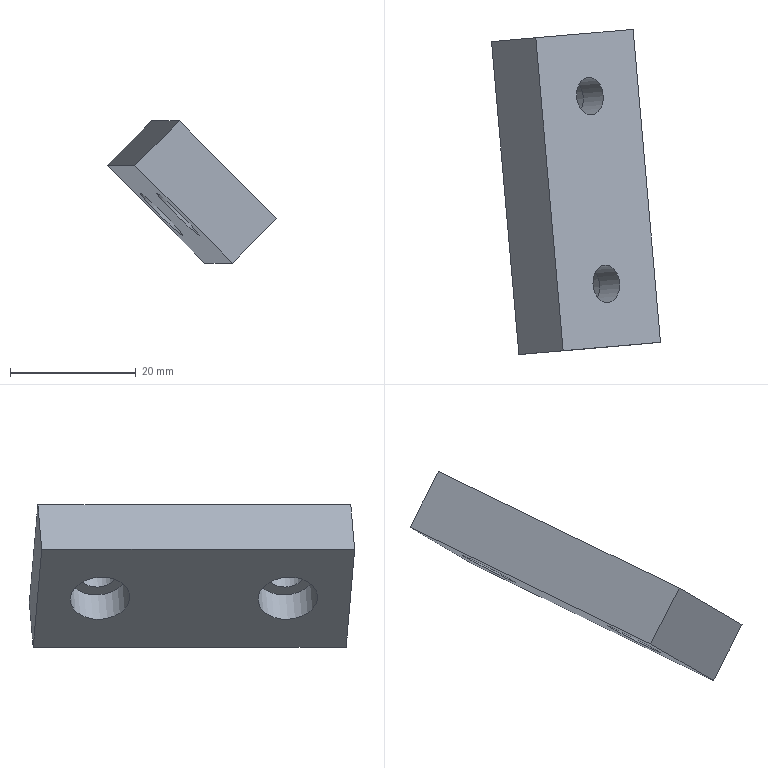Part | NX | features solid 2 | 1 solid | 12 faces | box 26.899 x 51.782 x 22.627 mm | volume 9966 mm3 | plane 8 | cylinder 4 | commonest cylinder face diameters 6 x2 9.5 x2
STEP:
#1=CARTESIAN_POINT('',(-359.245,41.849,8.934));
#2=VERTEX_POINT('',#1);
#3=CARTESIAN_POINT('',(-366.289,41.233,1.863));
#4=VERTEX_POINT('',#3);
#5=CARTESIAN_POINT('',(-359.245,41.849,8.934));
#6=DIRECTION('',(0.7044,0.06163,0.7071));
#7=VECTOR('',#6,1000.);
#8=LINE('',#5,#7);
#9=EDGE_CURVE('',#2,#4,#8,.F.);
#10=ORIENTED_EDGE('',*,*,#9,.F.);
#11=CARTESIAN_POINT('',(-354.887,-7.961,8.934));
#12=VERTEX_POINT('',#11);
#13=CARTESIAN_POINT('',(-359.463,44.34,8.934));
#14=DIRECTION('',(0.08716,-0.9962,0.));
#15=VECTOR('',#14,1000.);
#16=LINE('',#13,#15);
#17=EDGE_CURVE('',#2,#12,#16,.T.);
#18=ORIENTED_EDGE('',*,*,#17,.T.);
#19=CARTESIAN_POINT('',(-361.931,-8.577,1.863));
#20=VERTEX_POINT('',#19);
#21=CARTESIAN_POINT('',(-354.887,-7.961,8.934));
#22=DIRECTION('',(-0.7044,-0.06163,-0.7071));
#23=VECTOR('',#22,1000.);
#24=LINE('',#21,#23);
#25=EDGE_CURVE('',#12,#20,#24,.T.);
#26=ORIENTED_EDGE('',*,*,#25,.T.);
#27=CARTESIAN_POINT('',(-366.507,43.723,1.863));
#28=DIRECTION('',(0.08716,-0.9962,0.));
#29=VECTOR('',#28,1000.);
#30=LINE('',#27,#29);
#31=EDGE_CURVE('',#4,#20,#30,.T.);
#32=ORIENTED_EDGE('',*,*,#31,.F.);
#33=EDGE_LOOP('',(#10,#18,#26,#32));
#34=FACE_BOUND('',#33,.T.);
#35=CARTESIAN_POINT('',(-359.463,44.34,8.934));
#36=DIRECTION('',(0.7044,0.06163,-0.7071));
#37=DIRECTION('',(0.08716,-0.9962,0.));
#38=AXIS2_PLACEMENT_3D('',#35,#36,#37);
#39=PLANE('',#38);
#40=ADVANCED_FACE('',(#34),#39,.T.);
#41=ORIENTED_EDGE('',*,*,#25,.F.);
#42=CARTESIAN_POINT('',(-370.384,-9.317,24.49));
#43=VERTEX_POINT('',#42);
#44=CARTESIAN_POINT('',(-354.887,-7.961,8.934));
#45=DIRECTION('',(-0.7044,-0.06163,0.7071));
#46=VECTOR('',#45,1000.);
#47=LINE('',#44,#46);
#48=EDGE_CURVE('',#12,#43,#47,.T.);
#49=ORIENTED_EDGE('',*,*,#48,.T.);
#50=CARTESIAN_POINT('',(-377.428,-9.933,17.419));
#51=VERTEX_POINT('',#50);
#52=CARTESIAN_POINT('',(-370.384,-9.317,24.49));
#53=DIRECTION('',(0.7044,0.06163,0.7071));
#54=VECTOR('',#53,1000.);
#55=LINE('',#52,#54);
#56=EDGE_CURVE('',#43,#51,#55,.F.);
#57=ORIENTED_EDGE('',*,*,#56,.T.);
#58=CARTESIAN_POINT('',(-361.931,-8.577,1.863));
#59=DIRECTION('',(-0.7044,-0.06163,0.7071));
#60=VECTOR('',#59,1000.);
#61=LINE('',#58,#60);
#62=EDGE_CURVE('',#20,#51,#61,.T.);
#63=ORIENTED_EDGE('',*,*,#62,.F.);
#64=EDGE_LOOP('',(#41,#49,#57,#63));
#65=FACE_BOUND('',#64,.T.);
#66=CARTESIAN_POINT('',(-354.887,-7.961,8.934));
#67=DIRECTION('',(0.08716,-0.9962,0.));
#68=DIRECTION('',(-0.7044,-0.06163,0.7071));
#69=AXIS2_PLACEMENT_3D('',#66,#67,#68);
#70=PLANE('',#69);
#71=ADVANCED_FACE('',(#65),#70,.T.);
#72=ORIENTED_EDGE('',*,*,#56,.F.);
#73=CARTESIAN_POINT('',(-374.742,40.493,24.49));
#74=VERTEX_POINT('',#73);
#75=CARTESIAN_POINT('',(-374.96,42.984,24.49));
#76=DIRECTION('',(0.08716,-0.9962,0.));
#77=VECTOR('',#76,1000.);
#78=LINE('',#75,#77);
#79=EDGE_CURVE('',#74,#43,#78,.T.);
#80=ORIENTED_EDGE('',*,*,#79,.F.);
#81=CARTESIAN_POINT('',(-381.786,39.877,17.419));
#82=VERTEX_POINT('',#81);
#83=CARTESIAN_POINT('',(-374.742,40.493,24.49));
#84=DIRECTION('',(-0.7044,-0.06163,-0.7071));
#85=VECTOR('',#84,1000.);
#86=LINE('',#83,#85);
#87=EDGE_CURVE('',#74,#82,#86,.T.);
#88=ORIENTED_EDGE('',*,*,#87,.T.);
#89=CARTESIAN_POINT('',(-382.004,42.367,17.419));
#90=DIRECTION('',(0.08716,-0.9962,0.));
#91=VECTOR('',#90,1000.);
#92=LINE('',#89,#91);
#93=EDGE_CURVE('',#82,#51,#92,.T.);
#94=ORIENTED_EDGE('',*,*,#93,.T.);
#95=EDGE_LOOP('',(#72,#80,#88,#94));
#96=FACE_BOUND('',#95,.T.);
#97=CARTESIAN_POINT('',(-374.96,42.984,24.49));
#98=DIRECTION('',(0.7044,0.06163,-0.7071));
#99=DIRECTION('',(0.08716,-0.9962,0.));
#100=AXIS2_PLACEMENT_3D('',#97,#98,#99);
#101=PLANE('',#100);
#102=ADVANCED_FACE('',(#96),#101,.F.);
#103=CARTESIAN_POINT('',(-376.531,30.593,12.993));
#104=VERTEX_POINT('',#103);
#105=CARTESIAN_POINT('',(-373.166,30.593,9.641));
#106=DIRECTION('',(-0.7044,-0.06163,-0.7071));
#107=DIRECTION('',(-0.7085,0.,0.7058));
#108=AXIS2_PLACEMENT_3D('',#105,#106,#107);
#109=CIRCLE('',#108,4.75);
#110=EDGE_CURVE('',#104,#104,#109,.T.);
#111=ORIENTED_EDGE('',*,*,#110,.F.);
#112=EDGE_LOOP('',(#111));
#113=FACE_BOUND('',#112,.T.);
#114=CARTESIAN_POINT('',(-373.916,0.707,12.993));
#115=VERTEX_POINT('',#114);
#116=CARTESIAN_POINT('',(-370.551,0.707,9.641));
#117=DIRECTION('',(-0.7044,-0.06163,-0.7071));
#118=DIRECTION('',(-0.7085,0.,0.7058));
#119=AXIS2_PLACEMENT_3D('',#116,#117,#118);
#120=CIRCLE('',#119,4.75);
#121=EDGE_CURVE('',#115,#115,#120,.T.);
#122=ORIENTED_EDGE('',*,*,#121,.F.);
#123=EDGE_LOOP('',(#122));
#124=FACE_BOUND('',#123,.T.);
#125=ORIENTED_EDGE('',*,*,#93,.F.);
#126=CARTESIAN_POINT('',(-366.289,41.233,1.863));
#127=DIRECTION('',(0.7044,0.06163,-0.7071));
#128=VECTOR('',#127,1000.);
#129=LINE('',#126,#128);
#130=EDGE_CURVE('',#4,#82,#129,.F.);
#131=ORIENTED_EDGE('',*,*,#130,.F.);
#132=ORIENTED_EDGE('',*,*,#31,.T.);
#133=ORIENTED_EDGE('',*,*,#62,.T.);
#134=EDGE_LOOP('',(#125,#131,#132,#133));
#135=FACE_BOUND('',#134,.T.);
#136=CARTESIAN_POINT('',(-366.507,43.723,1.863));
#137=DIRECTION('',(-0.7044,-0.06163,-0.7071));
#138=DIRECTION('',(-0.7085,0.,0.7058));
#139=AXIS2_PLACEMENT_3D('',#136,#137,#138);
#140=PLANE('',#139);
#141=ADVANCED_FACE('',(#113,#124,#135),#140,.T.);
#142=CARTESIAN_POINT('',(-359.245,41.849,8.934));
#143=DIRECTION('',(0.7044,0.06163,-0.7071));
#144=VECTOR('',#143,1000.);
#145=LINE('',#142,#144);
#146=EDGE_CURVE('',#2,#74,#145,.F.);
#147=ORIENTED_EDGE('',*,*,#146,.F.);
#148=ORIENTED_EDGE('',*,*,#9,.T.);
#149=ORIENTED_EDGE('',*,*,#130,.T.);
#150=ORIENTED_EDGE('',*,*,#87,.F.);
#151=EDGE_LOOP('',(#147,#148,#149,#150));
#152=FACE_BOUND('',#151,.T.);
#153=CARTESIAN_POINT('',(-359.245,41.849,8.934));
#154=DIRECTION('',(0.08716,-0.9962,0.));
#155=DIRECTION('',(-0.7044,-0.06163,0.7071));
#156=AXIS2_PLACEMENT_3D('',#153,#154,#155);
#157=PLANE('',#156);
#158=ADVANCED_FACE('',(#152),#157,.F.);
#159=CARTESIAN_POINT('',(-368.247,31.209,18.829));
#160=VERTEX_POINT('',#159);
#161=CARTESIAN_POINT('',(-366.122,31.209,16.712));
#162=DIRECTION('',(-0.7044,-0.06163,-0.7071));
#163=DIRECTION('',(-0.7085,0.,0.7058));
#164=AXIS2_PLACEMENT_3D('',#161,#162,#163);
#165=CIRCLE('',#164,3.);
#166=EDGE_CURVE('',#160,#160,#165,.T.);
#167=ORIENTED_EDGE('',*,*,#166,.T.);
#168=EDGE_LOOP('',(#167));
#169=FACE_BOUND('',#168,.T.);
#170=CARTESIAN_POINT('',(-365.632,1.323,18.829));
#171=VERTEX_POINT('',#170);
#172=CARTESIAN_POINT('',(-363.507,1.323,16.712));
#173=DIRECTION('',(-0.7044,-0.06163,-0.7071));
#174=DIRECTION('',(-0.7085,0.,0.7058));
#175=AXIS2_PLACEMENT_3D('',#172,#173,#174);
#176=CIRCLE('',#175,3.);
#177=EDGE_CURVE('',#171,#171,#176,.T.);
#178=ORIENTED_EDGE('',*,*,#177,.T.);
#179=EDGE_LOOP('',(#178));
#180=FACE_BOUND('',#179,.T.);
#181=ORIENTED_EDGE('',*,*,#79,.T.);
#182=ORIENTED_EDGE('',*,*,#48,.F.);
#183=ORIENTED_EDGE('',*,*,#17,.F.);
#184=ORIENTED_EDGE('',*,*,#146,.T.);
#185=EDGE_LOOP('',(#181,#182,#183,#184));
#186=FACE_BOUND('',#185,.T.);
#187=CARTESIAN_POINT('',(-359.463,44.34,8.934));
#188=DIRECTION('',(-0.7044,-0.06163,-0.7071));
#189=DIRECTION('',(-0.7085,0.,0.7058));
#190=AXIS2_PLACEMENT_3D('',#187,#188,#189);
#191=PLANE('',#190);
#192=ADVANCED_FACE('',(#169,#180,#186),#191,.F.);
#193=CARTESIAN_POINT('',(-364.552,1.046,11.413));
#194=VERTEX_POINT('',#193);
#195=CARTESIAN_POINT('',(-366.677,1.046,13.53));
#196=DIRECTION('',(0.7044,0.06163,0.7071));
#197=DIRECTION('',(0.7085,0.,-0.7058));
#198=AXIS2_PLACEMENT_3D('',#195,#196,#197);
#199=CIRCLE('',#198,3.);
#200=EDGE_CURVE('',#194,#194,#199,.F.);
#201=ORIENTED_EDGE('',*,*,#200,.T.);
#202=EDGE_LOOP('',(#201));
#203=FACE_BOUND('',#202,.T.);
#204=ORIENTED_EDGE('',*,*,#177,.F.);
#205=EDGE_LOOP('',(#204));
#206=FACE_BOUND('',#205,.T.);
#207=CARTESIAN_POINT('',(-360.337,1.601,19.894));
#208=DIRECTION('',(-0.7044,-0.06163,-0.7071));
#209=DIRECTION('',(-0.7085,0.,0.7058));
#210=AXIS2_PLACEMENT_3D('',#207,#208,#209);
#211=CYLINDRICAL_SURFACE('',#210,3.);
#212=ADVANCED_FACE('',(#203,#206),#211,.F.);
#213=ORIENTED_EDGE('',*,*,#200,.F.);
#214=EDGE_LOOP('',(#213));
#215=FACE_BOUND('',#214,.T.);
#216=CARTESIAN_POINT('',(-370.042,1.046,16.882));
#217=VERTEX_POINT('',#216);
#218=CARTESIAN_POINT('',(-366.677,1.046,13.53));
#219=DIRECTION('',(-0.7044,-0.06163,-0.7071));
#220=DIRECTION('',(-0.7085,0.,0.7058));
#221=AXIS2_PLACEMENT_3D('',#218,#219,#220);
#222=CIRCLE('',#221,4.75);
#223=EDGE_CURVE('',#217,#217,#222,.T.);
#224=ORIENTED_EDGE('',*,*,#223,.T.);
#225=EDGE_LOOP('',(#224));
#226=FACE_BOUND('',#225,.T.);
#227=CARTESIAN_POINT('',(-366.677,1.046,13.53));
#228=DIRECTION('',(0.7044,0.06163,0.7071));
#229=DIRECTION('',(0.7085,0.,-0.7058));
#230=AXIS2_PLACEMENT_3D('',#227,#228,#229);
#231=PLANE('',#230);
#232=ADVANCED_FACE('',(#215,#226),#231,.F.);
#233=ORIENTED_EDGE('',*,*,#121,.T.);
#234=EDGE_LOOP('',(#233));
#235=FACE_BOUND('',#234,.T.);
#236=ORIENTED_EDGE('',*,*,#223,.F.);
#237=EDGE_LOOP('',(#236));
#238=FACE_BOUND('',#237,.T.);
#239=CARTESIAN_POINT('',(-366.677,1.046,13.53));
#240=DIRECTION('',(-0.7044,-0.06163,-0.7071));
#241=DIRECTION('',(-0.7085,0.,0.7058));
#242=AXIS2_PLACEMENT_3D('',#239,#240,#241);
#243=CYLINDRICAL_SURFACE('',#242,4.75);
#244=ADVANCED_FACE('',(#235,#238),#243,.F.);
#245=CARTESIAN_POINT('',(-367.166,30.932,11.413));
#246=VERTEX_POINT('',#245);
#247=CARTESIAN_POINT('',(-369.292,30.932,13.53));
#248=DIRECTION('',(0.7044,0.06163,0.7071));
#249=DIRECTION('',(0.7085,0.,-0.7058));
#250=AXIS2_PLACEMENT_3D('',#247,#248,#249);
#251=CIRCLE('',#250,3.);
#252=EDGE_CURVE('',#246,#246,#251,.F.);
#253=ORIENTED_EDGE('',*,*,#252,.T.);
#254=EDGE_LOOP('',(#253));
#255=FACE_BOUND('',#254,.T.);
#256=ORIENTED_EDGE('',*,*,#166,.F.);
#257=EDGE_LOOP('',(#256));
#258=FACE_BOUND('',#257,.T.);
#259=CARTESIAN_POINT('',(-362.952,31.486,19.894));
#260=DIRECTION('',(-0.7044,-0.06163,-0.7071));
#261=DIRECTION('',(-0.7085,0.,0.7058));
#262=AXIS2_PLACEMENT_3D('',#259,#260,#261);
#263=CYLINDRICAL_SURFACE('',#262,3.);
#264=ADVANCED_FACE('',(#255,#258),#263,.F.);
#265=ORIENTED_EDGE('',*,*,#252,.F.);
#266=EDGE_LOOP('',(#265));
#267=FACE_BOUND('',#266,.T.);
#268=CARTESIAN_POINT('',(-372.657,30.932,16.882));
#269=VERTEX_POINT('',#268);
#270=CARTESIAN_POINT('',(-369.292,30.932,13.53));
#271=DIRECTION('',(-0.7044,-0.06163,-0.7071));
#272=DIRECTION('',(-0.7085,0.,0.7058));
#273=AXIS2_PLACEMENT_3D('',#270,#271,#272);
#274=CIRCLE('',#273,4.75);
#275=EDGE_CURVE('',#269,#269,#274,.T.);
#276=ORIENTED_EDGE('',*,*,#275,.T.);
#277=EDGE_LOOP('',(#276));
#278=FACE_BOUND('',#277,.T.);
#279=CARTESIAN_POINT('',(-369.292,30.932,13.53));
#280=DIRECTION('',(0.7044,0.06163,0.7071));
#281=DIRECTION('',(0.7085,0.,-0.7058));
#282=AXIS2_PLACEMENT_3D('',#279,#280,#281);
#283=PLANE('',#282);
#284=ADVANCED_FACE('',(#267,#278),#283,.F.);
#285=ORIENTED_EDGE('',*,*,#110,.T.);
#286=EDGE_LOOP('',(#285));
#287=FACE_BOUND('',#286,.T.);
#288=ORIENTED_EDGE('',*,*,#275,.F.);
#289=EDGE_LOOP('',(#288));
#290=FACE_BOUND('',#289,.T.);
#291=CARTESIAN_POINT('',(-369.292,30.932,13.53));
#292=DIRECTION('',(-0.7044,-0.06163,-0.7071));
#293=DIRECTION('',(-0.7085,0.,0.7058));
#294=AXIS2_PLACEMENT_3D('',#291,#292,#293);
#295=CYLINDRICAL_SURFACE('',#294,4.75);
#296=ADVANCED_FACE('',(#287,#290),#295,.F.);
#297=CLOSED_SHELL('',(#40,#71,#102,#141,#158,#192,#212,#232,#244,#264,#284,#296));
#298=MANIFOLD_SOLID_BREP('',#297);
#299=(LENGTH_UNIT()NAMED_UNIT(*)SI_UNIT(.MILLI.,.METRE.));
#300=UNCERTAINTY_MEASURE_WITH_UNIT(LENGTH_MEASURE(0.00001),#299,'','');
#301=(NAMED_UNIT(*)PLANE_ANGLE_UNIT()SI_UNIT($,.RADIAN.));
#302=(NAMED_UNIT(*)SI_UNIT($,.STERADIAN.)SOLID_ANGLE_UNIT());
#303=(GEOMETRIC_REPRESENTATION_CONTEXT(3)GLOBAL_UNCERTAINTY_ASSIGNED_CONTEXT((#300))GLOBAL_UNIT_ASSIGNED_CONTEXT((#299,#301,#302))REPRESENTATION_CONTEXT('',''));
#304=ADVANCED_BREP_SHAPE_REPRESENTATION('',(#298),#303);